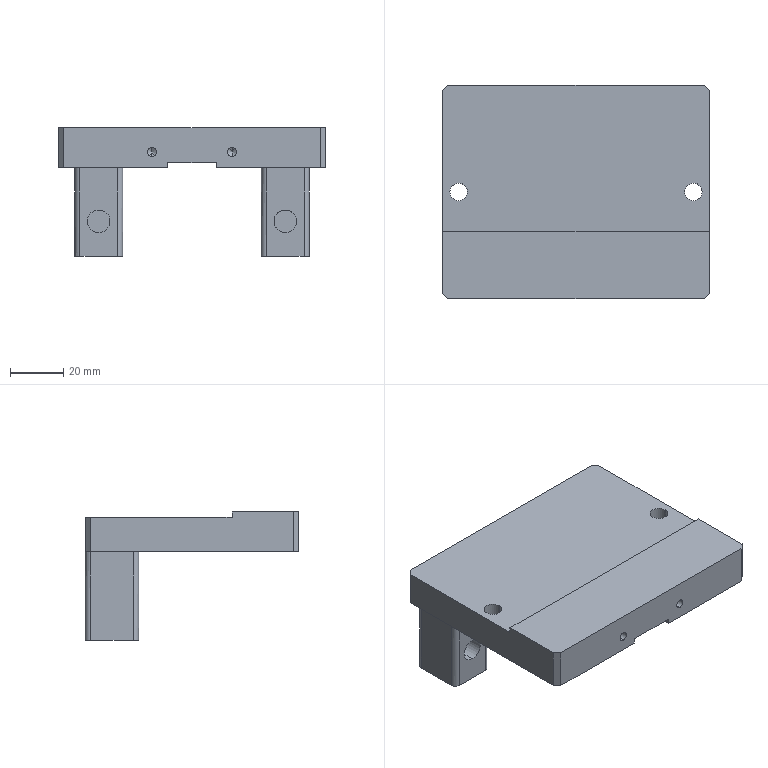Part | 1 solid | 76 faces | box 100 x 80 x 48 mm | volume 126220 mm3 | cylinder 34 | plane 28 | cone 14 | commonest cylinder face diameters 3.3 x8 4 x8 2.5 x6 6.6 x4 8.5 x4 11 x4